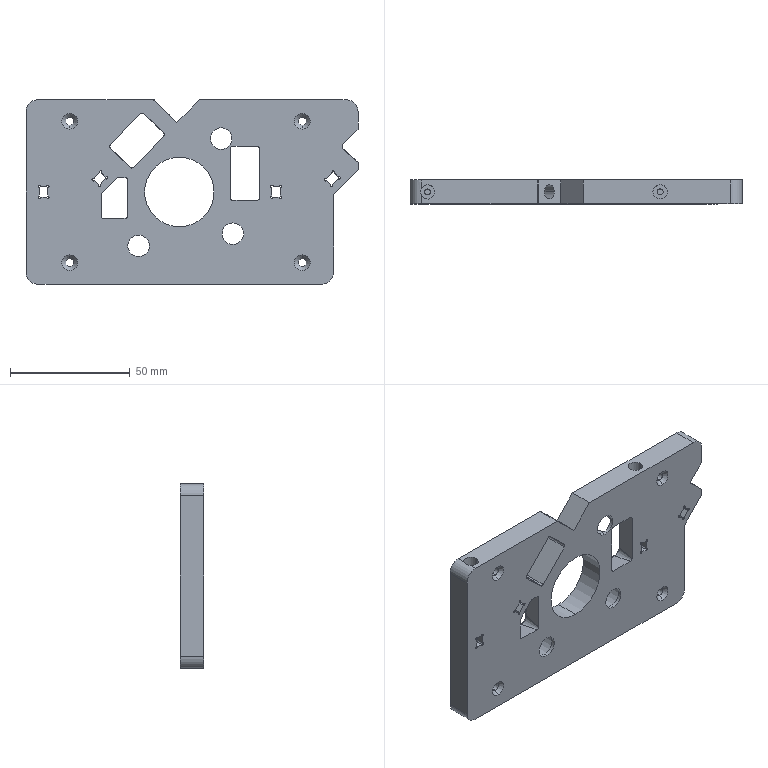Part | STEP file | 03-05 cutter fixing plate | 1 solid | 178 faces | box 138.5 x 10 x 77 mm | volume 77712 mm3 | cylinder 95 | plane 58 | cone 17 | torus 8 | commonest cylinder face diameters 1 x30 2 x16 6 x14 2.5 x8 3.4 x8 15 x7